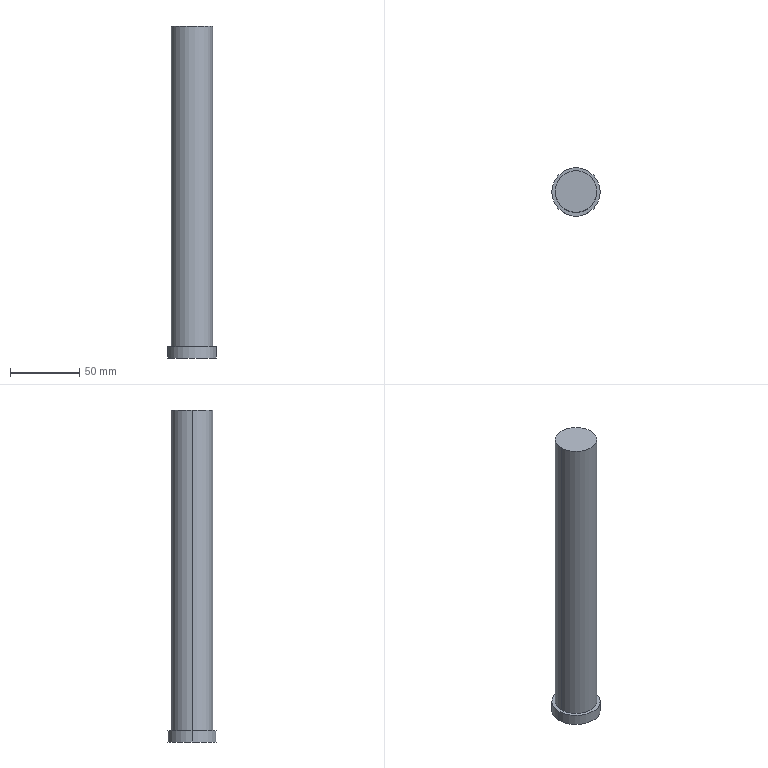Part | Creo | 1 solid | 7 faces | box 35 x 35 x 240 mm | volume 171688 mm3 | cylinder 4 | plane 3 | commonest cylinder face diameters 30 x2 35 x2
STEP:
#1=CARTESIAN_POINT('',(-182.5,365.,-227.5));
#2=VERTEX_POINT('',#1);
#3=CARTESIAN_POINT('',(-147.5,365.,-227.5));
#4=VERTEX_POINT('',#3);
#5=CARTESIAN_POINT('',(-165.,365.,-227.5));
#6=DIRECTION('',(0.,0.,1.));
#7=DIRECTION('',(-1.,0.,0.));
#8=AXIS2_PLACEMENT_3D('',#5,#6,#7);
#9=CIRCLE('',#8,17.5);
#10=EDGE_CURVE('',#2,#4,#9,.T.);
#11=ORIENTED_EDGE('',*,*,#10,.T.);
#12=CARTESIAN_POINT('',(-147.5,365.,-235.5));
#13=VERTEX_POINT('',#12);
#14=CARTESIAN_POINT('',(-147.5,365.,-227.5));
#15=DIRECTION('',(0.,0.,-1.));
#16=VECTOR('',#15,8.);
#17=LINE('',#14,#16);
#18=EDGE_CURVE('',#4,#13,#17,.T.);
#19=ORIENTED_EDGE('',*,*,#18,.T.);
#20=CARTESIAN_POINT('',(-182.5,365.,-235.5));
#21=VERTEX_POINT('',#20);
#22=CARTESIAN_POINT('',(-165.,365.,-235.5));
#23=DIRECTION('',(0.,0.,-1.));
#24=DIRECTION('',(1.,0.,0.));
#25=AXIS2_PLACEMENT_3D('',#22,#23,#24);
#26=CIRCLE('',#25,17.5);
#27=EDGE_CURVE('',#13,#21,#26,.T.);
#28=ORIENTED_EDGE('',*,*,#27,.T.);
#29=CARTESIAN_POINT('',(-182.5,365.,-227.5));
#30=DIRECTION('',(0.,0.,-1.));
#31=VECTOR('',#30,8.);
#32=LINE('',#29,#31);
#33=EDGE_CURVE('',#2,#21,#32,.T.);
#34=ORIENTED_EDGE('',*,*,#33,.F.);
#35=EDGE_LOOP('',(#11,#19,#28,#34));
#36=FACE_OUTER_BOUND('',#35,.F.);
#37=CARTESIAN_POINT('',(-165.,365.,-227.5));
#38=DIRECTION('',(0.,0.,-1.));
#39=DIRECTION('',(1.,0.,0.));
#40=AXIS2_PLACEMENT_3D('',#37,#38,#39);
#41=CYLINDRICAL_SURFACE('',#40,17.5);
#42=ADVANCED_FACE('',(#36),#41,.T.);
#43=CARTESIAN_POINT('',(-165.,365.,-227.5));
#44=DIRECTION('',(0.,0.,1.));
#45=DIRECTION('',(1.,0.,0.));
#46=AXIS2_PLACEMENT_3D('',#43,#44,#45);
#47=CIRCLE('',#46,17.5);
#48=EDGE_CURVE('',#4,#2,#47,.T.);
#49=ORIENTED_EDGE('',*,*,#48,.F.);
#50=ORIENTED_EDGE('',*,*,#10,.F.);
#51=EDGE_LOOP('',(#49,#50));
#52=FACE_OUTER_BOUND('',#51,.F.);
#53=CARTESIAN_POINT('',(-180.,365.,-227.5));
#54=VERTEX_POINT('',#53);
#55=CARTESIAN_POINT('',(-150.,365.,-227.5));
#56=VERTEX_POINT('',#55);
#57=CARTESIAN_POINT('',(-165.,365.,-227.5));
#58=DIRECTION('',(0.,0.,-1.));
#59=DIRECTION('',(-1.,0.,0.));
#60=AXIS2_PLACEMENT_3D('',#57,#58,#59);
#61=CIRCLE('',#60,15.);
#62=EDGE_CURVE('',#54,#56,#61,.T.);
#63=ORIENTED_EDGE('',*,*,#62,.F.);
#64=CARTESIAN_POINT('',(-165.,365.,-227.5));
#65=DIRECTION('',(0.,0.,-1.));
#66=DIRECTION('',(1.,0.,0.));
#67=AXIS2_PLACEMENT_3D('',#64,#65,#66);
#68=CIRCLE('',#67,15.);
#69=EDGE_CURVE('',#56,#54,#68,.T.);
#70=ORIENTED_EDGE('',*,*,#69,.F.);
#71=EDGE_LOOP('',(#63,#70));
#72=FACE_BOUND('',#71,.F.);
#73=CARTESIAN_POINT('',(-165.,365.,-227.5));
#74=DIRECTION('',(0.,0.,-1.));
#75=DIRECTION('',(1.,0.,0.));
#76=AXIS2_PLACEMENT_3D('',#73,#74,#75);
#77=PLANE('',#76);
#78=ADVANCED_FACE('',(#52,#72),#77,.F.);
#79=CARTESIAN_POINT('',(-150.,365.,4.5));
#80=VERTEX_POINT('',#79);
#81=CARTESIAN_POINT('',(-180.,365.,4.5));
#82=VERTEX_POINT('',#81);
#83=CARTESIAN_POINT('',(-165.,365.,4.5));
#84=DIRECTION('',(0.,0.,1.));
#85=DIRECTION('',(1.,0.,0.));
#86=AXIS2_PLACEMENT_3D('',#83,#84,#85);
#87=CIRCLE('',#86,15.);
#88=EDGE_CURVE('',#80,#82,#87,.T.);
#89=ORIENTED_EDGE('',*,*,#88,.T.);
#90=CARTESIAN_POINT('',(-180.,365.,-227.5));
#91=DIRECTION('',(0.,0.,1.));
#92=VECTOR('',#91,232.);
#93=LINE('',#90,#92);
#94=EDGE_CURVE('',#54,#82,#93,.T.);
#95=ORIENTED_EDGE('',*,*,#94,.F.);
#96=ORIENTED_EDGE('',*,*,#62,.T.);
#97=CARTESIAN_POINT('',(-150.,365.,-227.5));
#98=DIRECTION('',(0.,0.,1.));
#99=VECTOR('',#98,232.);
#100=LINE('',#97,#99);
#101=EDGE_CURVE('',#56,#80,#100,.T.);
#102=ORIENTED_EDGE('',*,*,#101,.T.);
#103=EDGE_LOOP('',(#89,#95,#96,#102));
#104=FACE_OUTER_BOUND('',#103,.F.);
#105=CARTESIAN_POINT('',(-165.,365.,-227.5));
#106=DIRECTION('',(0.,0.,1.));
#107=DIRECTION('',(-1.,0.,0.));
#108=AXIS2_PLACEMENT_3D('',#105,#106,#107);
#109=CYLINDRICAL_SURFACE('',#108,15.);
#110=ADVANCED_FACE('',(#104),#109,.T.);
#111=CARTESIAN_POINT('',(-165.,365.,4.5));
#112=DIRECTION('',(0.,0.,1.));
#113=DIRECTION('',(-1.,0.,0.));
#114=AXIS2_PLACEMENT_3D('',#111,#112,#113);
#115=CIRCLE('',#114,15.);
#116=EDGE_CURVE('',#82,#80,#115,.T.);
#117=ORIENTED_EDGE('',*,*,#116,.F.);
#118=ORIENTED_EDGE('',*,*,#88,.F.);
#119=EDGE_LOOP('',(#117,#118));
#120=FACE_OUTER_BOUND('',#119,.F.);
#121=CARTESIAN_POINT('',(-165.,365.,4.5));
#122=DIRECTION('',(0.,0.,1.));
#123=DIRECTION('',(-1.,0.,0.));
#124=AXIS2_PLACEMENT_3D('',#121,#122,#123);
#125=PLANE('',#124);
#126=ADVANCED_FACE('',(#120),#125,.T.);
#127=ORIENTED_EDGE('',*,*,#116,.T.);
#128=ORIENTED_EDGE('',*,*,#101,.F.);
#129=ORIENTED_EDGE('',*,*,#69,.T.);
#130=ORIENTED_EDGE('',*,*,#94,.T.);
#131=EDGE_LOOP('',(#127,#128,#129,#130));
#132=FACE_OUTER_BOUND('',#131,.F.);
#133=CARTESIAN_POINT('',(-165.,365.,-227.5));
#134=DIRECTION('',(0.,0.,1.));
#135=DIRECTION('',(-1.,0.,0.));
#136=AXIS2_PLACEMENT_3D('',#133,#134,#135);
#137=CYLINDRICAL_SURFACE('',#136,15.);
#138=ADVANCED_FACE('',(#132),#137,.T.);
#139=ORIENTED_EDGE('',*,*,#48,.T.);
#140=ORIENTED_EDGE('',*,*,#33,.T.);
#141=CARTESIAN_POINT('',(-165.,365.,-235.5));
#142=DIRECTION('',(0.,0.,-1.));
#143=DIRECTION('',(-1.,0.,0.));
#144=AXIS2_PLACEMENT_3D('',#141,#142,#143);
#145=CIRCLE('',#144,17.5);
#146=EDGE_CURVE('',#21,#13,#145,.T.);
#147=ORIENTED_EDGE('',*,*,#146,.T.);
#148=ORIENTED_EDGE('',*,*,#18,.F.);
#149=EDGE_LOOP('',(#139,#140,#147,#148));
#150=FACE_OUTER_BOUND('',#149,.F.);
#151=CARTESIAN_POINT('',(-165.,365.,-227.5));
#152=DIRECTION('',(0.,0.,-1.));
#153=DIRECTION('',(1.,0.,0.));
#154=AXIS2_PLACEMENT_3D('',#151,#152,#153);
#155=CYLINDRICAL_SURFACE('',#154,17.5);
#156=ADVANCED_FACE('',(#150),#155,.T.);
#157=ORIENTED_EDGE('',*,*,#27,.F.);
#158=ORIENTED_EDGE('',*,*,#146,.F.);
#159=EDGE_LOOP('',(#157,#158));
#160=FACE_OUTER_BOUND('',#159,.F.);
#161=CARTESIAN_POINT('',(-165.,365.,-235.5));
#162=DIRECTION('',(0.,0.,-1.));
#163=DIRECTION('',(1.,0.,0.));
#164=AXIS2_PLACEMENT_3D('',#161,#162,#163);
#165=PLANE('',#164);
#166=ADVANCED_FACE('',(#160),#165,.T.);
#167=CLOSED_SHELL('',(#42,#78,#110,#126,#138,#156,#166));
#168=MANIFOLD_SOLID_BREP('',#167);
#169=(LENGTH_UNIT()NAMED_UNIT(*)SI_UNIT(.MILLI.,.METRE.));
#170=UNCERTAINTY_MEASURE_WITH_UNIT(LENGTH_MEASURE(0.0245),#169,'','');
#171=(NAMED_UNIT(*)PLANE_ANGLE_UNIT()SI_UNIT($,.RADIAN.));
#172=PLANE_ANGLE_MEASURE_WITH_UNIT(PLANE_ANGLE_MEASURE(0.01745),#171);
#173=(CONVERSION_BASED_UNIT('DEGREE',#172)NAMED_UNIT(*)PLANE_ANGLE_UNIT());
#174=(NAMED_UNIT(*)SI_UNIT($,.STERADIAN.)SOLID_ANGLE_UNIT());
#175=(GEOMETRIC_REPRESENTATION_CONTEXT(3)GLOBAL_UNCERTAINTY_ASSIGNED_CONTEXT((#170))GLOBAL_UNIT_ASSIGNED_CONTEXT((#169,#173,#174))REPRESENTATION_CONTEXT('',''));
#176=ADVANCED_BREP_SHAPE_REPRESENTATION('',(#168),#175);